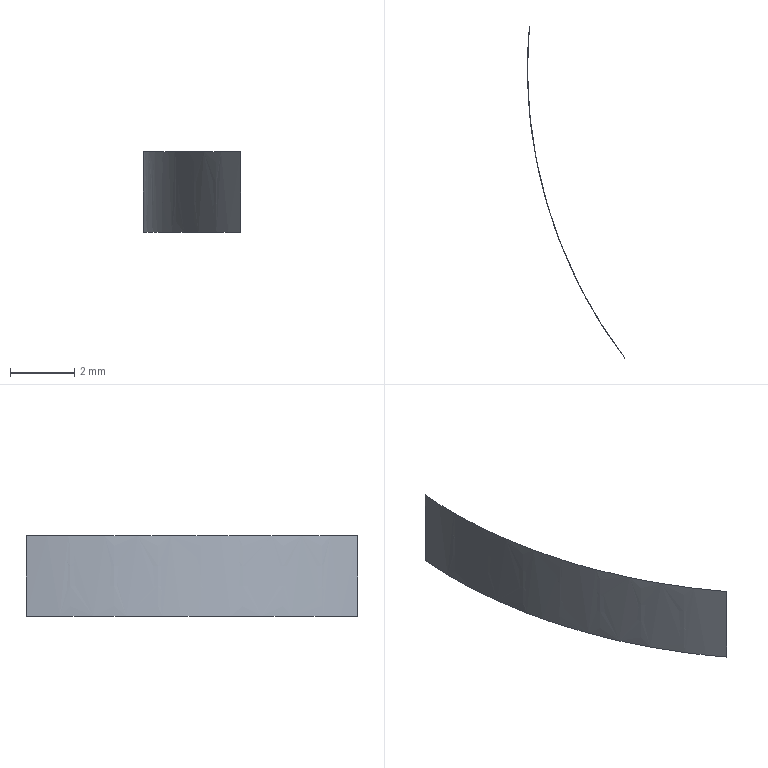Part | STEP file | lll_id386_x_t | 1 solid | 2 faces | box 3.021 x 10.335 x 2.5 mm | volume 0.02061 mm3 | other 1 | cylinder 1 | commonest cylinder face diameters 30 x1